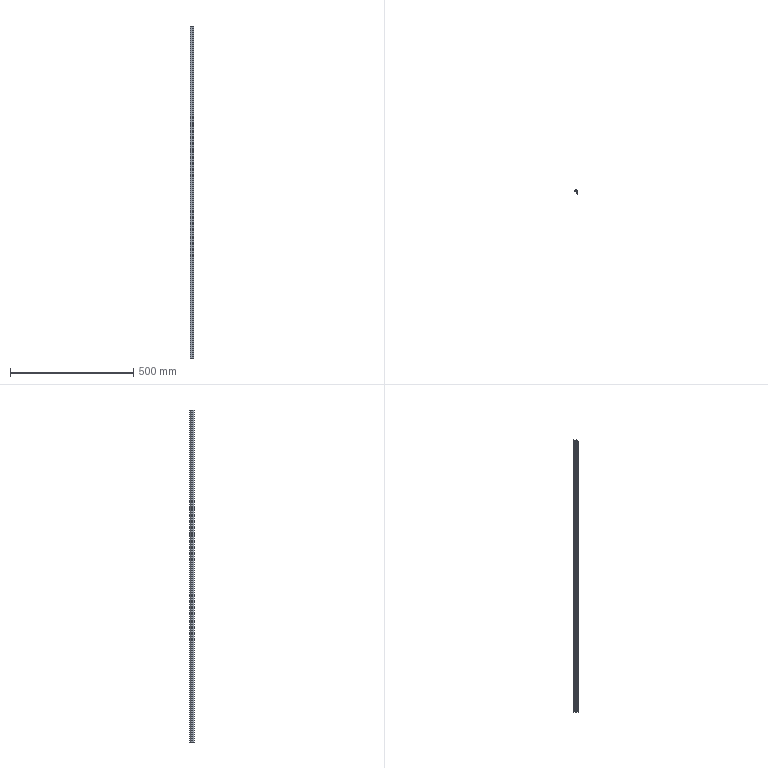Part | SolidWorks | features BaseBody 1, ICE 1, MoveFace 1 | 1 solid | 27 faces | box 14 x 20.3 x 1348 mm | volume 68634 mm3 | plane 20 | cylinder 7 | commonest cylinder face diameters 0.387 x2 0.8 x2 0.4 x1 20 x1 22 x1
STEP:
#1=CARTESIAN_POINT('',(-5.304,-0.625,200.));
#2=VERTEX_POINT('',#1);
#3=CARTESIAN_POINT('',(-5.449,-0.8125,200.));
#4=VERTEX_POINT('',#3);
#5=CARTESIAN_POINT('',(-5.255,-0.8125,200.));
#6=DIRECTION('',(0.,0.,1.));
#7=DIRECTION('',(-1.,0.,0.));
#8=AXIS2_PLACEMENT_3D('',#5,#6,#7);
#9=CIRCLE('',#8,0.1937);
#10=EDGE_CURVE('',#2,#4,#9,.T.);
#11=ORIENTED_EDGE('',*,*,#10,.T.);
#12=CARTESIAN_POINT('',(-5.449,-0.8125,-1148.));
#13=VERTEX_POINT('',#12);
#14=CARTESIAN_POINT('',(-5.449,-0.8125,230.));
#15=DIRECTION('',(0.,0.,-1.));
#16=VECTOR('',#15,1000.);
#17=LINE('',#14,#16);
#18=EDGE_CURVE('',#4,#13,#17,.T.);
#19=ORIENTED_EDGE('',*,*,#18,.T.);
#20=CARTESIAN_POINT('',(-5.304,-0.625,-1148.));
#21=VERTEX_POINT('',#20);
#22=CARTESIAN_POINT('',(-5.255,-0.8125,-1148.));
#23=DIRECTION('',(0.,0.,-1.));
#24=DIRECTION('',(1.,0.,0.));
#25=AXIS2_PLACEMENT_3D('',#22,#23,#24);
#26=CIRCLE('',#25,0.1937);
#27=EDGE_CURVE('',#13,#21,#26,.T.);
#28=ORIENTED_EDGE('',*,*,#27,.T.);
#29=CARTESIAN_POINT('',(-5.304,-0.625,230.));
#30=DIRECTION('',(0.,0.,-1.));
#31=VECTOR('',#30,1000.);
#32=LINE('',#29,#31);
#33=EDGE_CURVE('',#2,#21,#32,.T.);
#34=ORIENTED_EDGE('',*,*,#33,.F.);
#35=EDGE_LOOP('',(#11,#19,#28,#34));
#36=FACE_OUTER_BOUND('',#35,.T.);
#37=CARTESIAN_POINT('',(-5.255,-0.8125,230.));
#38=DIRECTION('',(0.,0.,-1.));
#39=DIRECTION('',(-1.,0.,0.));
#40=AXIS2_PLACEMENT_3D('',#37,#38,#39);
#41=CYLINDRICAL_SURFACE('',#40,0.1937);
#42=ADVANCED_FACE('',(#36),#41,.F.);
#43=CARTESIAN_POINT('',(5.,-1.,-1148.));
#44=VERTEX_POINT('',#43);
#45=CARTESIAN_POINT('',(5.,-14.3,-1148.));
#46=VERTEX_POINT('',#45);
#47=CARTESIAN_POINT('',(5.,29.623,-1148.));
#48=DIRECTION('',(0.,-1.,0.));
#49=VECTOR('',#48,1000.);
#50=LINE('',#47,#49);
#51=EDGE_CURVE('',#44,#46,#50,.T.);
#52=ORIENTED_EDGE('',*,*,#51,.F.);
#53=CARTESIAN_POINT('',(5.,-1.,200.));
#54=VERTEX_POINT('',#53);
#55=CARTESIAN_POINT('',(5.,-1.,230.));
#56=DIRECTION('',(0.,0.,-1.));
#57=VECTOR('',#56,1000.);
#58=LINE('',#55,#57);
#59=EDGE_CURVE('',#54,#44,#58,.T.);
#60=ORIENTED_EDGE('',*,*,#59,.F.);
#61=CARTESIAN_POINT('',(5.,-14.3,200.));
#62=VERTEX_POINT('',#61);
#63=CARTESIAN_POINT('',(5.,-14.3,200.));
#64=DIRECTION('',(0.,1.,0.));
#65=VECTOR('',#64,1000.);
#66=LINE('',#63,#65);
#67=EDGE_CURVE('',#62,#54,#66,.T.);
#68=ORIENTED_EDGE('',*,*,#67,.F.);
#69=CARTESIAN_POINT('',(5.,-14.3,230.));
#70=DIRECTION('',(0.,0.,1.));
#71=VECTOR('',#70,1000.);
#72=LINE('',#69,#71);
#73=EDGE_CURVE('',#46,#62,#72,.T.);
#74=ORIENTED_EDGE('',*,*,#73,.F.);
#75=EDGE_LOOP('',(#52,#60,#68,#74));
#76=FACE_OUTER_BOUND('',#75,.T.);
#77=CARTESIAN_POINT('',(5.,-14.3,230.));
#78=DIRECTION('',(-1.,0.,0.));
#79=DIRECTION('',(0.,0.,1.));
#80=AXIS2_PLACEMENT_3D('',#77,#78,#79);
#81=PLANE('',#80);
#82=ADVANCED_FACE('',(#76),#81,.F.);
#83=CARTESIAN_POINT('',(-9.,-2.,-1148.));
#84=VERTEX_POINT('',#83);
#85=CARTESIAN_POINT('',(-9.,-2.,200.));
#86=VERTEX_POINT('',#85);
#87=CARTESIAN_POINT('',(-9.,-2.,230.));
#88=DIRECTION('',(0.,0.,1.));
#89=VECTOR('',#88,1000.);
#90=LINE('',#87,#89);
#91=EDGE_CURVE('',#84,#86,#90,.T.);
#92=ORIENTED_EDGE('',*,*,#91,.F.);
#93=CARTESIAN_POINT('',(0.9,-2.,-1148.));
#94=VERTEX_POINT('',#93);
#95=CARTESIAN_POINT('',(5.,-2.,-1148.));
#96=DIRECTION('',(-1.,0.,0.));
#97=VECTOR('',#96,1000.);
#98=LINE('',#95,#97);
#99=EDGE_CURVE('',#94,#84,#98,.T.);
#100=ORIENTED_EDGE('',*,*,#99,.F.);
#101=CARTESIAN_POINT('',(0.9,-2.,200.));
#102=VERTEX_POINT('',#101);
#103=CARTESIAN_POINT('',(0.9,-2.,230.));
#104=DIRECTION('',(0.,0.,-1.));
#105=VECTOR('',#104,1000.);
#106=LINE('',#103,#105);
#107=EDGE_CURVE('',#102,#94,#106,.T.);
#108=ORIENTED_EDGE('',*,*,#107,.F.);
#109=CARTESIAN_POINT('',(5.,-2.,200.));
#110=DIRECTION('',(1.,0.,0.));
#111=VECTOR('',#110,1000.);
#112=LINE('',#109,#111);
#113=EDGE_CURVE('',#86,#102,#112,.T.);
#114=ORIENTED_EDGE('',*,*,#113,.F.);
#115=EDGE_LOOP('',(#92,#100,#108,#114));
#116=FACE_OUTER_BOUND('',#115,.T.);
#117=CARTESIAN_POINT('',(-9.,-2.,230.));
#118=DIRECTION('',(0.,1.,0.));
#119=DIRECTION('',(0.,0.,1.));
#120=AXIS2_PLACEMENT_3D('',#117,#118,#119);
#121=PLANE('',#120);
#122=ADVANCED_FACE('',(#116),#121,.F.);
#123=CARTESIAN_POINT('',(4.,-6.,200.));
#124=VERTEX_POINT('',#123);
#125=CARTESIAN_POINT('',(4.,-3.,200.));
#126=VERTEX_POINT('',#125);
#127=CARTESIAN_POINT('',(4.,29.623,200.));
#128=DIRECTION('',(0.,1.,0.));
#129=VECTOR('',#128,1000.);
#130=LINE('',#127,#129);
#131=EDGE_CURVE('',#124,#126,#130,.T.);
#132=ORIENTED_EDGE('',*,*,#131,.F.);
#133=CARTESIAN_POINT('',(1.,-6.,200.));
#134=VERTEX_POINT('',#133);
#135=CARTESIAN_POINT('',(5.,-6.,200.));
#136=DIRECTION('',(1.,0.,0.));
#137=VECTOR('',#136,1000.);
#138=LINE('',#135,#137);
#139=EDGE_CURVE('',#134,#124,#138,.T.);
#140=ORIENTED_EDGE('',*,*,#139,.F.);
#141=CARTESIAN_POINT('',(1.,-6.7,200.));
#142=VERTEX_POINT('',#141);
#143=CARTESIAN_POINT('',(1.,-6.,200.));
#144=DIRECTION('',(0.,-1.,0.));
#145=VECTOR('',#144,1000.);
#146=LINE('',#143,#145);
#147=EDGE_CURVE('',#134,#142,#146,.T.);
#148=ORIENTED_EDGE('',*,*,#147,.T.);
#149=CARTESIAN_POINT('',(-1.7,-6.7,200.));
#150=VERTEX_POINT('',#149);
#151=CARTESIAN_POINT('',(5.,-6.7,200.));
#152=DIRECTION('',(1.,0.,0.));
#153=VECTOR('',#152,1000.);
#154=LINE('',#151,#153);
#155=EDGE_CURVE('',#150,#142,#154,.T.);
#156=ORIENTED_EDGE('',*,*,#155,.F.);
#157=CARTESIAN_POINT('',(-1.7,-7.7,200.));
#158=VERTEX_POINT('',#157);
#159=CARTESIAN_POINT('',(-1.7,-6.7,200.));
#160=DIRECTION('',(0.,-1.,0.));
#161=VECTOR('',#160,1000.);
#162=LINE('',#159,#161);
#163=EDGE_CURVE('',#150,#158,#162,.T.);
#164=ORIENTED_EDGE('',*,*,#163,.T.);
#165=CARTESIAN_POINT('',(4.,-7.7,200.));
#166=VERTEX_POINT('',#165);
#167=CARTESIAN_POINT('',(5.,-7.7,200.));
#168=DIRECTION('',(-1.,0.,0.));
#169=VECTOR('',#168,1000.);
#170=LINE('',#167,#169);
#171=EDGE_CURVE('',#166,#158,#170,.T.);
#172=ORIENTED_EDGE('',*,*,#171,.F.);
#173=CARTESIAN_POINT('',(4.,-14.3,200.));
#174=VERTEX_POINT('',#173);
#175=CARTESIAN_POINT('',(4.,29.623,200.));
#176=DIRECTION('',(0.,1.,0.));
#177=VECTOR('',#176,1000.);
#178=LINE('',#175,#177);
#179=EDGE_CURVE('',#174,#166,#178,.T.);
#180=ORIENTED_EDGE('',*,*,#179,.F.);
#181=CARTESIAN_POINT('',(5.,-14.3,200.));
#182=DIRECTION('',(-1.,0.,0.));
#183=VECTOR('',#182,1000.);
#184=LINE('',#181,#183);
#185=EDGE_CURVE('',#62,#174,#184,.T.);
#186=ORIENTED_EDGE('',*,*,#185,.F.);
#187=ORIENTED_EDGE('',*,*,#67,.T.);
#188=CARTESIAN_POINT('',(-5.207,-1.,200.));
#189=VERTEX_POINT('',#188);
#190=CARTESIAN_POINT('',(5.,-1.,200.));
#191=DIRECTION('',(1.,0.,0.));
#192=VECTOR('',#191,1000.);
#193=LINE('',#190,#192);
#194=EDGE_CURVE('',#189,#54,#193,.T.);
#195=ORIENTED_EDGE('',*,*,#194,.F.);
#196=CARTESIAN_POINT('',(-5.255,-0.8125,200.));
#197=DIRECTION('',(0.,0.,1.));
#198=DIRECTION('',(-1.,0.,0.));
#199=AXIS2_PLACEMENT_3D('',#196,#197,#198);
#200=CIRCLE('',#199,0.1937);
#201=EDGE_CURVE('',#4,#189,#200,.T.);
#202=ORIENTED_EDGE('',*,*,#201,.F.);
#203=ORIENTED_EDGE('',*,*,#10,.F.);
#204=CARTESIAN_POINT('',(-1.368,3.063,200.));
#205=VERTEX_POINT('',#204);
#206=CARTESIAN_POINT('',(-10.628,9.,200.));
#207=DIRECTION('',(0.,0.,1.));
#208=DIRECTION('',(-1.,0.,0.));
#209=AXIS2_PLACEMENT_3D('',#206,#207,#208);
#210=CIRCLE('',#209,11.);
#211=EDGE_CURVE('',#2,#205,#210,.T.);
#212=ORIENTED_EDGE('',*,*,#211,.T.);
#213=CARTESIAN_POINT('',(-1.,2.955,200.));
#214=VERTEX_POINT('',#213);
#215=CARTESIAN_POINT('',(-1.2,2.955,200.));
#216=DIRECTION('',(0.,0.,1.));
#217=DIRECTION('',(-1.,0.,0.));
#218=AXIS2_PLACEMENT_3D('',#215,#216,#217);
#219=CIRCLE('',#218,0.2);
#220=EDGE_CURVE('',#214,#205,#219,.T.);
#221=ORIENTED_EDGE('',*,*,#220,.F.);
#222=CARTESIAN_POINT('',(-1.,1.5,200.));
#223=VERTEX_POINT('',#222);
#224=CARTESIAN_POINT('',(-1.,2.955,200.));
#225=DIRECTION('',(0.,1.,0.));
#226=VECTOR('',#225,1000.);
#227=LINE('',#224,#226);
#228=EDGE_CURVE('',#223,#214,#227,.T.);
#229=ORIENTED_EDGE('',*,*,#228,.F.);
#230=CARTESIAN_POINT('',(0.,1.5,200.));
#231=VERTEX_POINT('',#230);
#232=CARTESIAN_POINT('',(-1.,1.5,200.));
#233=DIRECTION('',(-1.,0.,0.));
#234=VECTOR('',#233,1000.);
#235=LINE('',#232,#234);
#236=EDGE_CURVE('',#231,#223,#235,.T.);
#237=ORIENTED_EDGE('',*,*,#236,.F.);
#238=CARTESIAN_POINT('',(0.,6.,200.));
#239=VERTEX_POINT('',#238);
#240=CARTESIAN_POINT('',(0.,1.5,200.));
#241=DIRECTION('',(0.,-1.,0.));
#242=VECTOR('',#241,1000.);
#243=LINE('',#240,#242);
#244=EDGE_CURVE('',#239,#231,#243,.T.);
#245=ORIENTED_EDGE('',*,*,#244,.F.);
#246=CARTESIAN_POINT('',(-0.8,6.,200.));
#247=VERTEX_POINT('',#246);
#248=CARTESIAN_POINT('',(0.,6.,200.));
#249=DIRECTION('',(1.,0.,0.));
#250=VECTOR('',#249,1000.);
#251=LINE('',#248,#250);
#252=EDGE_CURVE('',#247,#239,#251,.T.);
#253=ORIENTED_EDGE('',*,*,#252,.F.);
#254=CARTESIAN_POINT('',(-1.178,5.731,200.));
#255=VERTEX_POINT('',#254);
#256=CARTESIAN_POINT('',(-0.8,5.6,200.));
#257=DIRECTION('',(0.,0.,1.));
#258=DIRECTION('',(-1.,0.,0.));
#259=AXIS2_PLACEMENT_3D('',#256,#257,#258);
#260=CIRCLE('',#259,0.4);
#261=EDGE_CURVE('',#247,#255,#260,.T.);
#262=ORIENTED_EDGE('',*,*,#261,.T.);
#263=CARTESIAN_POINT('',(-8.678,-0.8077,200.));
#264=VERTEX_POINT('',#263);
#265=CARTESIAN_POINT('',(-10.628,9.,200.));
#266=DIRECTION('',(0.,0.,1.));
#267=DIRECTION('',(-1.,0.,0.));
#268=AXIS2_PLACEMENT_3D('',#265,#266,#267);
#269=CIRCLE('',#268,10.);
#270=EDGE_CURVE('',#264,#255,#269,.T.);
#271=ORIENTED_EDGE('',*,*,#270,.F.);
#272=CARTESIAN_POINT('',(-9.,-1.2,200.));
#273=VERTEX_POINT('',#272);
#274=CARTESIAN_POINT('',(-8.6,-1.2,200.));
#275=DIRECTION('',(0.,0.,1.));
#276=DIRECTION('',(-1.,0.,0.));
#277=AXIS2_PLACEMENT_3D('',#274,#275,#276);
#278=CIRCLE('',#277,0.4);
#279=EDGE_CURVE('',#264,#273,#278,.T.);
#280=ORIENTED_EDGE('',*,*,#279,.T.);
#281=CARTESIAN_POINT('',(-9.,8.,200.));
#282=DIRECTION('',(0.,-1.,0.));
#283=VECTOR('',#282,1000.);
#284=LINE('',#281,#283);
#285=EDGE_CURVE('',#273,#86,#284,.T.);
#286=ORIENTED_EDGE('',*,*,#285,.T.);
#287=ORIENTED_EDGE('',*,*,#113,.T.);
#288=CARTESIAN_POINT('',(0.9,-3.,200.));
#289=VERTEX_POINT('',#288);
#290=CARTESIAN_POINT('',(0.9,29.623,200.));
#291=DIRECTION('',(0.,1.,0.));
#292=VECTOR('',#291,1000.);
#293=LINE('',#290,#292);
#294=EDGE_CURVE('',#289,#102,#293,.T.);
#295=ORIENTED_EDGE('',*,*,#294,.F.);
#296=CARTESIAN_POINT('',(5.,-3.,200.));
#297=DIRECTION('',(-1.,0.,0.));
#298=VECTOR('',#297,1000.);
#299=LINE('',#296,#298);
#300=EDGE_CURVE('',#126,#289,#299,.T.);
#301=ORIENTED_EDGE('',*,*,#300,.F.);
#302=EDGE_LOOP('',(#132,#140,#148,#156,#164,#172,#180,#186,#187,#195,#202,#203,#212,#221,#229,#237,#245,#253,#262,#271,#280,#286,#287,#295,#301));
#303=FACE_OUTER_BOUND('',#302,.T.);
#304=CARTESIAN_POINT('',(5.,29.623,200.));
#305=DIRECTION('',(0.,0.,-1.));
#306=DIRECTION('',(-1.,0.,0.));
#307=AXIS2_PLACEMENT_3D('',#304,#305,#306);
#308=PLANE('',#307);
#309=ADVANCED_FACE('',(#303),#308,.F.);
#310=ORIENTED_EDGE('',*,*,#185,.T.);
#311=CARTESIAN_POINT('',(4.,-14.3,-1148.));
#312=VERTEX_POINT('',#311);
#313=CARTESIAN_POINT('',(4.,-14.3,230.));
#314=DIRECTION('',(0.,0.,1.));
#315=VECTOR('',#314,1000.);
#316=LINE('',#313,#315);
#317=EDGE_CURVE('',#312,#174,#316,.T.);
#318=ORIENTED_EDGE('',*,*,#317,.F.);
#319=CARTESIAN_POINT('',(5.,-14.3,-1148.));
#320=DIRECTION('',(-1.,0.,0.));
#321=VECTOR('',#320,1000.);
#322=LINE('',#319,#321);
#323=EDGE_CURVE('',#46,#312,#322,.T.);
#324=ORIENTED_EDGE('',*,*,#323,.F.);
#325=ORIENTED_EDGE('',*,*,#73,.T.);
#326=EDGE_LOOP('',(#310,#318,#324,#325));
#327=FACE_OUTER_BOUND('',#326,.T.);
#328=CARTESIAN_POINT('',(4.,-14.3,230.));
#329=DIRECTION('',(0.,1.,0.));
#330=DIRECTION('',(0.,0.,1.));
#331=AXIS2_PLACEMENT_3D('',#328,#329,#330);
#332=PLANE('',#331);
#333=ADVANCED_FACE('',(#327),#332,.F.);
#334=ORIENTED_EDGE('',*,*,#51,.T.);
#335=ORIENTED_EDGE('',*,*,#323,.T.);
#336=CARTESIAN_POINT('',(4.,-7.7,-1148.));
#337=VERTEX_POINT('',#336);
#338=CARTESIAN_POINT('',(4.,-7.7,-1148.));
#339=DIRECTION('',(0.,-1.,0.));
#340=VECTOR('',#339,1000.);
#341=LINE('',#338,#340);
#342=EDGE_CURVE('',#337,#312,#341,.T.);
#343=ORIENTED_EDGE('',*,*,#342,.F.);
#344=CARTESIAN_POINT('',(-1.7,-7.7,-1148.));
#345=VERTEX_POINT('',#344);
#346=CARTESIAN_POINT('',(-1.7,-7.7,-1148.));
#347=DIRECTION('',(1.,0.,0.));
#348=VECTOR('',#347,1000.);
#349=LINE('',#346,#348);
#350=EDGE_CURVE('',#345,#337,#349,.T.);
#351=ORIENTED_EDGE('',*,*,#350,.F.);
#352=CARTESIAN_POINT('',(-1.7,-6.7,-1148.));
#353=VERTEX_POINT('',#352);
#354=CARTESIAN_POINT('',(-1.7,29.623,-1148.));
#355=DIRECTION('',(0.,1.,0.));
#356=VECTOR('',#355,1000.);
#357=LINE('',#354,#356);
#358=EDGE_CURVE('',#345,#353,#357,.T.);
#359=ORIENTED_EDGE('',*,*,#358,.T.);
#360=CARTESIAN_POINT('',(1.,-6.7,-1148.));
#361=VERTEX_POINT('',#360);
#362=CARTESIAN_POINT('',(1.,-6.7,-1148.));
#363=DIRECTION('',(-1.,0.,0.));
#364=VECTOR('',#363,1000.);
#365=LINE('',#362,#364);
#366=EDGE_CURVE('',#361,#353,#365,.T.);
#367=ORIENTED_EDGE('',*,*,#366,.F.);
#368=CARTESIAN_POINT('',(1.,-6.,-1148.));
#369=VERTEX_POINT('',#368);
#370=CARTESIAN_POINT('',(1.,29.623,-1148.));
#371=DIRECTION('',(0.,1.,0.));
#372=VECTOR('',#371,1000.);
#373=LINE('',#370,#372);
#374=EDGE_CURVE('',#361,#369,#373,.T.);
#375=ORIENTED_EDGE('',*,*,#374,.T.);
#376=CARTESIAN_POINT('',(4.,-6.,-1148.));
#377=VERTEX_POINT('',#376);
#378=CARTESIAN_POINT('',(4.,-6.,-1148.));
#379=DIRECTION('',(-1.,0.,0.));
#380=VECTOR('',#379,1000.);
#381=LINE('',#378,#380);
#382=EDGE_CURVE('',#377,#369,#381,.T.);
#383=ORIENTED_EDGE('',*,*,#382,.F.);
#384=CARTESIAN_POINT('',(4.,-3.,-1148.));
#385=VERTEX_POINT('',#384);
#386=CARTESIAN_POINT('',(4.,-3.,-1148.));
#387=DIRECTION('',(0.,-1.,0.));
#388=VECTOR('',#387,1000.);
#389=LINE('',#386,#388);
#390=EDGE_CURVE('',#385,#377,#389,.T.);
#391=ORIENTED_EDGE('',*,*,#390,.F.);
#392=CARTESIAN_POINT('',(0.9,-3.,-1148.));
#393=VERTEX_POINT('',#392);
#394=CARTESIAN_POINT('',(0.9,-3.,-1148.));
#395=DIRECTION('',(1.,0.,0.));
#396=VECTOR('',#395,1000.);
#397=LINE('',#394,#396);
#398=EDGE_CURVE('',#393,#385,#397,.T.);
#399=ORIENTED_EDGE('',*,*,#398,.F.);
#400=CARTESIAN_POINT('',(0.9,-2.,-1148.));
#401=DIRECTION('',(0.,-1.,0.));
#402=VECTOR('',#401,1000.);
#403=LINE('',#400,#402);
#404=EDGE_CURVE('',#94,#393,#403,.T.);
#405=ORIENTED_EDGE('',*,*,#404,.F.);
#406=ORIENTED_EDGE('',*,*,#99,.T.);
#407=CARTESIAN_POINT('',(-9.,-1.2,-1148.));
#408=VERTEX_POINT('',#407);
#409=CARTESIAN_POINT('',(-9.,-1.2,-1148.));
#410=DIRECTION('',(0.,-1.,0.));
#411=VECTOR('',#410,1000.);
#412=LINE('',#409,#411);
#413=EDGE_CURVE('',#408,#84,#412,.T.);
#414=ORIENTED_EDGE('',*,*,#413,.F.);
#415=CARTESIAN_POINT('',(-8.678,-0.8077,-1148.));
#416=VERTEX_POINT('',#415);
#417=CARTESIAN_POINT('',(-8.6,-1.2,-1148.));
#418=DIRECTION('',(0.,0.,-1.));
#419=DIRECTION('',(1.,0.,0.));
#420=AXIS2_PLACEMENT_3D('',#417,#418,#419);
#421=CIRCLE('',#420,0.4);
#422=EDGE_CURVE('',#408,#416,#421,.T.);
#423=ORIENTED_EDGE('',*,*,#422,.T.);
#424=CARTESIAN_POINT('',(-1.178,5.731,-1148.));
#425=VERTEX_POINT('',#424);
#426=CARTESIAN_POINT('',(-10.628,9.,-1148.));
#427=DIRECTION('',(0.,0.,-1.));
#428=DIRECTION('',(1.,0.,0.));
#429=AXIS2_PLACEMENT_3D('',#426,#427,#428);
#430=CIRCLE('',#429,10.);
#431=EDGE_CURVE('',#425,#416,#430,.T.);
#432=ORIENTED_EDGE('',*,*,#431,.F.);
#433=CARTESIAN_POINT('',(-0.8,6.,-1148.));
#434=VERTEX_POINT('',#433);
#435=CARTESIAN_POINT('',(-0.8,5.6,-1148.));
#436=DIRECTION('',(0.,0.,-1.));
#437=DIRECTION('',(1.,0.,0.));
#438=AXIS2_PLACEMENT_3D('',#435,#436,#437);
#439=CIRCLE('',#438,0.4);
#440=EDGE_CURVE('',#425,#434,#439,.T.);
#441=ORIENTED_EDGE('',*,*,#440,.T.);
#442=CARTESIAN_POINT('',(0.,6.,-1148.));
#443=VERTEX_POINT('',#442);
#444=CARTESIAN_POINT('',(0.,6.,-1148.));
#445=DIRECTION('',(-1.,0.,0.));
#446=VECTOR('',#445,1000.);
#447=LINE('',#444,#446);
#448=EDGE_CURVE('',#443,#434,#447,.T.);
#449=ORIENTED_EDGE('',*,*,#448,.F.);
#450=CARTESIAN_POINT('',(0.,1.5,-1148.));
#451=VERTEX_POINT('',#450);
#452=CARTESIAN_POINT('',(0.,1.5,-1148.));
#453=DIRECTION('',(0.,1.,0.));
#454=VECTOR('',#453,1000.);
#455=LINE('',#452,#454);
#456=EDGE_CURVE('',#451,#443,#455,.T.);
#457=ORIENTED_EDGE('',*,*,#456,.F.);
#458=CARTESIAN_POINT('',(-1.,1.5,-1148.));
#459=VERTEX_POINT('',#458);
#460=CARTESIAN_POINT('',(-1.,1.5,-1148.));
#461=DIRECTION('',(1.,0.,0.));
#462=VECTOR('',#461,1000.);
#463=LINE('',#460,#462);
#464=EDGE_CURVE('',#459,#451,#463,.T.);
#465=ORIENTED_EDGE('',*,*,#464,.F.);
#466=CARTESIAN_POINT('',(-1.,2.955,-1148.));
#467=VERTEX_POINT('',#466);
#468=CARTESIAN_POINT('',(-1.,2.955,-1148.));
#469=DIRECTION('',(0.,-1.,0.));
#470=VECTOR('',#469,1000.);
#471=LINE('',#468,#470);
#472=EDGE_CURVE('',#467,#459,#471,.T.);
#473=ORIENTED_EDGE('',*,*,#472,.F.);
#474=CARTESIAN_POINT('',(-1.368,3.063,-1148.));
#475=VERTEX_POINT('',#474);
#476=CARTESIAN_POINT('',(-1.2,2.955,-1148.));
#477=DIRECTION('',(0.,0.,-1.));
#478=DIRECTION('',(1.,0.,0.));
#479=AXIS2_PLACEMENT_3D('',#476,#477,#478);
#480=CIRCLE('',#479,0.2);
#481=EDGE_CURVE('',#475,#467,#480,.T.);
#482=ORIENTED_EDGE('',*,*,#481,.F.);
#483=CARTESIAN_POINT('',(-10.628,9.,-1148.));
#484=DIRECTION('',(0.,0.,-1.));
#485=DIRECTION('',(1.,0.,0.));
#486=AXIS2_PLACEMENT_3D('',#483,#484,#485);
#487=CIRCLE('',#486,11.);
#488=EDGE_CURVE('',#475,#21,#487,.T.);
#489=ORIENTED_EDGE('',*,*,#488,.T.);
#490=ORIENTED_EDGE('',*,*,#27,.F.);
#491=CARTESIAN_POINT('',(-5.207,-1.,-1148.));
#492=VERTEX_POINT('',#491);
#493=CARTESIAN_POINT('',(-5.255,-0.8125,-1148.));
#494=DIRECTION('',(0.,0.,-1.));
#495=DIRECTION('',(1.,0.,0.));
#496=AXIS2_PLACEMENT_3D('',#493,#494,#495);
#497=CIRCLE('',#496,0.1937);
#498=EDGE_CURVE('',#492,#13,#497,.T.);
#499=ORIENTED_EDGE('',*,*,#498,.F.);
#500=CARTESIAN_POINT('',(5.,-1.,-1148.));
#501=DIRECTION('',(-1.,0.,0.));
#502=VECTOR('',#501,1000.);
#503=LINE('',#500,#502);
#504=EDGE_CURVE('',#44,#492,#503,.T.);
#505=ORIENTED_EDGE('',*,*,#504,.F.);
#506=EDGE_LOOP('',(#334,#335,#343,#351,#359,#367,#375,#383,#391,#399,#405,#406,#414,#423,#432,#441,#449,#457,#465,#473,#482,#489,#490,#499,#505));
#507=FACE_OUTER_BOUND('',#506,.T.);
#508=CARTESIAN_POINT('',(5.,29.623,-1148.));
#509=DIRECTION('',(0.,0.,1.));
#510=DIRECTION('',(1.,0.,0.));
#511=AXIS2_PLACEMENT_3D('',#508,#509,#510);
#512=PLANE('',#511);
#513=ADVANCED_FACE('',(#507),#512,.F.);
#514=ORIENTED_EDGE('',*,*,#59,.T.);
#515=ORIENTED_EDGE('',*,*,#504,.T.);
#516=CARTESIAN_POINT('',(-5.207,-1.,230.));
#517=DIRECTION('',(0.,0.,-1.));
#518=VECTOR('',#517,1000.);
#519=LINE('',#516,#518);
#520=EDGE_CURVE('',#189,#492,#519,.T.);
#521=ORIENTED_EDGE('',*,*,#520,.F.);
#522=ORIENTED_EDGE('',*,*,#194,.T.);
#523=EDGE_LOOP('',(#514,#515,#521,#522));
#524=FACE_OUTER_BOUND('',#523,.T.);
#525=CARTESIAN_POINT('',(5.,-1.,230.));
#526=DIRECTION('',(0.,-1.,0.));
#527=DIRECTION('',(0.,0.,-1.));
#528=AXIS2_PLACEMENT_3D('',#525,#526,#527);
#529=PLANE('',#528);
#530=ADVANCED_FACE('',(#524),#529,.F.);
#531=CARTESIAN_POINT('',(-9.,-1.2,230.));
#532=DIRECTION('',(0.,0.,1.));
#533=VECTOR('',#532,1000.);
#534=LINE('',#531,#533);
#535=EDGE_CURVE('',#408,#273,#534,.T.);
#536=ORIENTED_EDGE('',*,*,#535,.F.);
#537=ORIENTED_EDGE('',*,*,#413,.T.);
#538=ORIENTED_EDGE('',*,*,#91,.T.);
#539=ORIENTED_EDGE('',*,*,#285,.F.);
#540=EDGE_LOOP('',(#536,#537,#538,#539));
#541=FACE_OUTER_BOUND('',#540,.T.);
#542=CARTESIAN_POINT('',(-9.,-1.2,230.));
#543=DIRECTION('',(1.,0.,0.));
#544=DIRECTION('',(0.,0.,-1.));
#545=AXIS2_PLACEMENT_3D('',#542,#543,#544);
#546=PLANE('',#545);
#547=ADVANCED_FACE('',(#541),#546,.F.);
#548=ORIENTED_EDGE('',*,*,#294,.T.);
#549=ORIENTED_EDGE('',*,*,#107,.T.);
#550=ORIENTED_EDGE('',*,*,#404,.T.);
#551=CARTESIAN_POINT('',(0.9,-3.,230.));
#552=DIRECTION('',(0.,0.,-1.));
#553=VECTOR('',#552,1000.);
#554=LINE('',#551,#553);
#555=EDGE_CURVE('',#289,#393,#554,.T.);
#556=ORIENTED_EDGE('',*,*,#555,.F.);
#557=EDGE_LOOP('',(#548,#549,#550,#556));
#558=FACE_OUTER_BOUND('',#557,.T.);
#559=CARTESIAN_POINT('',(0.9,-2.,230.));
#560=DIRECTION('',(1.,0.,0.));
#561=DIRECTION('',(0.,0.,-1.));
#562=AXIS2_PLACEMENT_3D('',#559,#560,#561);
#563=PLANE('',#562);
#564=ADVANCED_FACE('',(#558),#563,.F.);
#565=ORIENTED_EDGE('',*,*,#300,.T.);
#566=ORIENTED_EDGE('',*,*,#555,.T.);
#567=ORIENTED_EDGE('',*,*,#398,.T.);
#568=CARTESIAN_POINT('',(4.,-3.,230.));
#569=DIRECTION('',(0.,0.,-1.));
#570=VECTOR('',#569,1000.);
#571=LINE('',#568,#570);
#572=EDGE_CURVE('',#126,#385,#571,.T.);
#573=ORIENTED_EDGE('',*,*,#572,.F.);
#574=EDGE_LOOP('',(#565,#566,#567,#573));
#575=FACE_OUTER_BOUND('',#574,.T.);
#576=CARTESIAN_POINT('',(0.9,-3.,230.));
#577=DIRECTION('',(0.,1.,0.));
#578=DIRECTION('',(0.,0.,1.));
#579=AXIS2_PLACEMENT_3D('',#576,#577,#578);
#580=PLANE('',#579);
#581=ADVANCED_FACE('',(#575),#580,.F.);
#582=ORIENTED_EDGE('',*,*,#131,.T.);
#583=ORIENTED_EDGE('',*,*,#572,.T.);
#584=ORIENTED_EDGE('',*,*,#390,.T.);
#585=CARTESIAN_POINT('',(4.,-6.,230.));
#586=DIRECTION('',(0.,0.,-1.));
#587=VECTOR('',#586,1000.);
#588=LINE('',#585,#587);
#589=EDGE_CURVE('',#124,#377,#588,.T.);
#590=ORIENTED_EDGE('',*,*,#589,.F.);
#591=EDGE_LOOP('',(#582,#583,#584,#590));
#592=FACE_OUTER_BOUND('',#591,.T.);
#593=CARTESIAN_POINT('',(4.,-3.,230.));
#594=DIRECTION('',(1.,0.,0.));
#595=DIRECTION('',(0.,0.,-1.));
#596=AXIS2_PLACEMENT_3D('',#593,#594,#595);
#597=PLANE('',#596);
#598=ADVANCED_FACE('',(#592),#597,.F.);
#599=ORIENTED_EDGE('',*,*,#139,.T.);
#600=ORIENTED_EDGE('',*,*,#589,.T.);
#601=ORIENTED_EDGE('',*,*,#382,.T.);
#602=CARTESIAN_POINT('',(1.,-6.,230.));
#603=DIRECTION('',(0.,0.,-1.));
#604=VECTOR('',#603,1000.);
#605=LINE('',#602,#604);
#606=EDGE_CURVE('',#134,#369,#605,.T.);
#607=ORIENTED_EDGE('',*,*,#606,.F.);
#608=EDGE_LOOP('',(#599,#600,#601,#607));
#609=FACE_OUTER_BOUND('',#608,.T.);
#610=CARTESIAN_POINT('',(4.,-6.,230.));
#611=DIRECTION('',(0.,-1.,0.));
#612=DIRECTION('',(0.,0.,-1.));
#613=AXIS2_PLACEMENT_3D('',#610,#611,#612);
#614=PLANE('',#613);
#615=ADVANCED_FACE('',(#609),#614,.F.);
#616=ORIENTED_EDGE('',*,*,#155,.T.);
#617=CARTESIAN_POINT('',(1.,-6.7,230.));
#618=DIRECTION('',(0.,0.,1.));
#619=VECTOR('',#618,1000.);
#620=LINE('',#617,#619);
#621=EDGE_CURVE('',#361,#142,#620,.T.);
#622=ORIENTED_EDGE('',*,*,#621,.F.);
#623=ORIENTED_EDGE('',*,*,#366,.T.);
#624=CARTESIAN_POINT('',(-1.7,-6.7,230.));
#625=DIRECTION('',(0.,0.,-1.));
#626=VECTOR('',#625,1000.);
#627=LINE('',#624,#626);
#628=EDGE_CURVE('',#150,#353,#627,.T.);
#629=ORIENTED_EDGE('',*,*,#628,.F.);
#630=EDGE_LOOP('',(#616,#622,#623,#629));
#631=FACE_OUTER_BOUND('',#630,.T.);
#632=CARTESIAN_POINT('',(1.,-6.7,230.));
#633=DIRECTION('',(0.,-1.,0.));
#634=DIRECTION('',(0.,0.,-1.));
#635=AXIS2_PLACEMENT_3D('',#632,#633,#634);
#636=PLANE('',#635);
#637=ADVANCED_FACE('',(#631),#636,.F.);
#638=ORIENTED_EDGE('',*,*,#171,.T.);
#639=CARTESIAN_POINT('',(-1.7,-7.7,230.));
#640=DIRECTION('',(0.,0.,1.));
#641=VECTOR('',#640,1000.);
#642=LINE('',#639,#641);
#643=EDGE_CURVE('',#345,#158,#642,.T.);
#644=ORIENTED_EDGE('',*,*,#643,.F.);
#645=ORIENTED_EDGE('',*,*,#350,.T.);
#646=CARTESIAN_POINT('',(4.,-7.7,230.));
#647=DIRECTION('',(0.,0.,-1.));
#648=VECTOR('',#647,1000.);
#649=LINE('',#646,#648);
#650=EDGE_CURVE('',#166,#337,#649,.T.);
#651=ORIENTED_EDGE('',*,*,#650,.F.);
#652=EDGE_LOOP('',(#638,#644,#645,#651));
#653=FACE_OUTER_BOUND('',#652,.T.);
#654=CARTESIAN_POINT('',(-1.7,-7.7,230.));
#655=DIRECTION('',(0.,1.,0.));
#656=DIRECTION('',(0.,0.,1.));
#657=AXIS2_PLACEMENT_3D('',#654,#655,#656);
#658=PLANE('',#657);
#659=ADVANCED_FACE('',(#653),#658,.F.);
#660=ORIENTED_EDGE('',*,*,#179,.T.);
#661=ORIENTED_EDGE('',*,*,#650,.T.);
#662=ORIENTED_EDGE('',*,*,#342,.T.);
#663=ORIENTED_EDGE('',*,*,#317,.T.);
#664=EDGE_LOOP('',(#660,#661,#662,#663));
#665=FACE_OUTER_BOUND('',#664,.T.);
#666=CARTESIAN_POINT('',(4.,-7.7,230.));
#667=DIRECTION('',(1.,0.,0.));
#668=DIRECTION('',(0.,0.,-1.));
#669=AXIS2_PLACEMENT_3D('',#666,#667,#668);
#670=PLANE('',#669);
#671=ADVANCED_FACE('',(#665),#670,.F.);
#672=ORIENTED_EDGE('',*,*,#18,.F.);
#673=ORIENTED_EDGE('',*,*,#201,.T.);
#674=ORIENTED_EDGE('',*,*,#520,.T.);
#675=ORIENTED_EDGE('',*,*,#498,.T.);
#676=EDGE_LOOP('',(#672,#673,#674,#675));
#677=FACE_OUTER_BOUND('',#676,.T.);
#678=CARTESIAN_POINT('',(-5.255,-0.8125,230.));
#679=DIRECTION('',(0.,0.,-1.));
#680=DIRECTION('',(-1.,0.,0.));
#681=AXIS2_PLACEMENT_3D('',#678,#679,#680);
#682=CYLINDRICAL_SURFACE('',#681,0.1937);
#683=ADVANCED_FACE('',(#677),#682,.F.);
#684=CARTESIAN_POINT('',(-1.,2.955,230.));
#685=DIRECTION('',(0.,0.,1.));
#686=VECTOR('',#685,1000.);
#687=LINE('',#684,#686);
#688=EDGE_CURVE('',#467,#214,#687,.T.);
#689=ORIENTED_EDGE('',*,*,#688,.F.);
#690=ORIENTED_EDGE('',*,*,#472,.T.);
#691=CARTESIAN_POINT('',(-1.,1.5,230.));
#692=DIRECTION('',(0.,0.,-1.));
#693=VECTOR('',#692,1000.);
#694=LINE('',#691,#693);
#695=EDGE_CURVE('',#223,#459,#694,.T.);
#696=ORIENTED_EDGE('',*,*,#695,.F.);
#697=ORIENTED_EDGE('',*,*,#228,.T.);
#698=EDGE_LOOP('',(#689,#690,#696,#697));
#699=FACE_OUTER_BOUND('',#698,.T.);
#700=CARTESIAN_POINT('',(-1.,2.955,230.));
#701=DIRECTION('',(1.,0.,0.));
#702=DIRECTION('',(0.,0.,-1.));
#703=AXIS2_PLACEMENT_3D('',#700,#701,#702);
#704=PLANE('',#703);
#705=ADVANCED_FACE('',(#699),#704,.F.);
#706=ORIENTED_EDGE('',*,*,#488,.F.);
#707=CARTESIAN_POINT('',(-1.368,3.063,230.));
#708=DIRECTION('',(0.,0.,1.));
#709=VECTOR('',#708,1000.);
#710=LINE('',#707,#709);
#711=EDGE_CURVE('',#475,#205,#710,.T.);
#712=ORIENTED_EDGE('',*,*,#711,.T.);
#713=ORIENTED_EDGE('',*,*,#211,.F.);
#714=ORIENTED_EDGE('',*,*,#33,.T.);
#715=EDGE_LOOP('',(#706,#712,#713,#714));
#716=FACE_OUTER_BOUND('',#715,.T.);
#717=CARTESIAN_POINT('',(-10.628,9.,230.));
#718=DIRECTION('',(0.,0.,-1.));
#719=DIRECTION('',(-1.,0.,0.));
#720=AXIS2_PLACEMENT_3D('',#717,#718,#719);
#721=CYLINDRICAL_SURFACE('',#720,11.);
#722=ADVANCED_FACE('',(#716),#721,.T.);
#723=CARTESIAN_POINT('',(-1.178,5.731,230.));
#724=DIRECTION('',(0.,0.,1.));
#725=VECTOR('',#724,1000.);
#726=LINE('',#723,#725);
#727=EDGE_CURVE('',#425,#255,#726,.T.);
#728=ORIENTED_EDGE('',*,*,#727,.F.);
#729=ORIENTED_EDGE('',*,*,#431,.T.);
#730=CARTESIAN_POINT('',(-8.678,-0.8077,230.));
#731=DIRECTION('',(0.,0.,-1.));
#732=VECTOR('',#731,1000.);
#733=LINE('',#730,#732);
#734=EDGE_CURVE('',#264,#416,#733,.T.);
#735=ORIENTED_EDGE('',*,*,#734,.F.);
#736=ORIENTED_EDGE('',*,*,#270,.T.);
#737=EDGE_LOOP('',(#728,#729,#735,#736));
#738=FACE_OUTER_BOUND('',#737,.T.);
#739=CARTESIAN_POINT('',(-10.628,9.,230.));
#740=DIRECTION('',(0.,0.,-1.));
#741=DIRECTION('',(-1.,0.,0.));
#742=AXIS2_PLACEMENT_3D('',#739,#740,#741);
#743=CYLINDRICAL_SURFACE('',#742,10.);
#744=ADVANCED_FACE('',(#738),#743,.F.);
#745=CARTESIAN_POINT('',(0.,1.5,230.));
#746=DIRECTION('',(0.,0.,1.));
#747=VECTOR('',#746,1000.);
#748=LINE('',#745,#747);
#749=EDGE_CURVE('',#451,#231,#748,.T.);
#750=ORIENTED_EDGE('',*,*,#749,.F.);
#751=ORIENTED_EDGE('',*,*,#456,.T.);
#752=CARTESIAN_POINT('',(0.,6.,230.));
#753=DIRECTION('',(0.,0.,-1.));
#754=VECTOR('',#753,1000.);
#755=LINE('',#752,#754);
#756=EDGE_CURVE('',#239,#443,#755,.T.);
#757=ORIENTED_EDGE('',*,*,#756,.F.);
#758=ORIENTED_EDGE('',*,*,#244,.T.);
#759=EDGE_LOOP('',(#750,#751,#757,#758));
#760=FACE_OUTER_BOUND('',#759,.T.);
#761=CARTESIAN_POINT('',(0.,1.5,230.));
#762=DIRECTION('',(-1.,0.,0.));
#763=DIRECTION('',(0.,0.,1.));
#764=AXIS2_PLACEMENT_3D('',#761,#762,#763);
#765=PLANE('',#764);
#766=ADVANCED_FACE('',(#760),#765,.F.);
#767=ORIENTED_EDGE('',*,*,#422,.F.);
#768=ORIENTED_EDGE('',*,*,#535,.T.);
#769=ORIENTED_EDGE('',*,*,#279,.F.);
#770=ORIENTED_EDGE('',*,*,#734,.T.);
#771=EDGE_LOOP('',(#767,#768,#769,#770));
#772=FACE_OUTER_BOUND('',#771,.T.);
#773=CARTESIAN_POINT('',(-8.6,-1.2,230.));
#774=DIRECTION('',(0.,0.,-1.));
#775=DIRECTION('',(-1.,0.,0.));
#776=AXIS2_PLACEMENT_3D('',#773,#774,#775);
#777=CYLINDRICAL_SURFACE('',#776,0.4);
#778=ADVANCED_FACE('',(#772),#777,.T.);
#779=ORIENTED_EDGE('',*,*,#147,.F.);
#780=ORIENTED_EDGE('',*,*,#606,.T.);
#781=ORIENTED_EDGE('',*,*,#374,.F.);
#782=ORIENTED_EDGE('',*,*,#621,.T.);
#783=EDGE_LOOP('',(#779,#780,#781,#782));
#784=FACE_OUTER_BOUND('',#783,.T.);
#785=CARTESIAN_POINT('',(1.,-6.,230.));
#786=DIRECTION('',(1.,0.,0.));
#787=DIRECTION('',(0.,0.,-1.));
#788=AXIS2_PLACEMENT_3D('',#785,#786,#787);
#789=PLANE('',#788);
#790=ADVANCED_FACE('',(#784),#789,.F.);
#791=ORIENTED_EDGE('',*,*,#163,.F.);
#792=ORIENTED_EDGE('',*,*,#628,.T.);
#793=ORIENTED_EDGE('',*,*,#358,.F.);
#794=ORIENTED_EDGE('',*,*,#643,.T.);
#795=EDGE_LOOP('',(#791,#792,#793,#794));
#796=FACE_OUTER_BOUND('',#795,.T.);
#797=CARTESIAN_POINT('',(-1.7,-6.7,230.));
#798=DIRECTION('',(1.,0.,0.));
#799=DIRECTION('',(0.,0.,-1.));
#800=AXIS2_PLACEMENT_3D('',#797,#798,#799);
#801=PLANE('',#800);
#802=ADVANCED_FACE('',(#796),#801,.F.);
#803=ORIENTED_EDGE('',*,*,#711,.F.);
#804=ORIENTED_EDGE('',*,*,#481,.T.);
#805=ORIENTED_EDGE('',*,*,#688,.T.);
#806=ORIENTED_EDGE('',*,*,#220,.T.);
#807=EDGE_LOOP('',(#803,#804,#805,#806));
#808=FACE_OUTER_BOUND('',#807,.T.);
#809=CARTESIAN_POINT('',(-1.2,2.955,230.));
#810=DIRECTION('',(0.,0.,-1.));
#811=DIRECTION('',(-1.,0.,0.));
#812=AXIS2_PLACEMENT_3D('',#809,#810,#811);
#813=CYLINDRICAL_SURFACE('',#812,0.2);
#814=ADVANCED_FACE('',(#808),#813,.F.);
#815=ORIENTED_EDGE('',*,*,#695,.T.);
#816=ORIENTED_EDGE('',*,*,#464,.T.);
#817=ORIENTED_EDGE('',*,*,#749,.T.);
#818=ORIENTED_EDGE('',*,*,#236,.T.);
#819=EDGE_LOOP('',(#815,#816,#817,#818));
#820=FACE_OUTER_BOUND('',#819,.T.);
#821=CARTESIAN_POINT('',(-1.,1.5,230.));
#822=DIRECTION('',(0.,1.,0.));
#823=DIRECTION('',(0.,0.,1.));
#824=AXIS2_PLACEMENT_3D('',#821,#822,#823);
#825=PLANE('',#824);
#826=ADVANCED_FACE('',(#820),#825,.F.);
#827=ORIENTED_EDGE('',*,*,#440,.F.);
#828=ORIENTED_EDGE('',*,*,#727,.T.);
#829=ORIENTED_EDGE('',*,*,#261,.F.);
#830=CARTESIAN_POINT('',(-0.8,6.,230.));
#831=DIRECTION('',(0.,0.,-1.));
#832=VECTOR('',#831,1000.);
#833=LINE('',#830,#832);
#834=EDGE_CURVE('',#247,#434,#833,.T.);
#835=ORIENTED_EDGE('',*,*,#834,.T.);
#836=EDGE_LOOP('',(#827,#828,#829,#835));
#837=FACE_OUTER_BOUND('',#836,.T.);
#838=CARTESIAN_POINT('',(-0.8,5.6,230.));
#839=DIRECTION('',(0.,0.,-1.));
#840=DIRECTION('',(-1.,0.,0.));
#841=AXIS2_PLACEMENT_3D('',#838,#839,#840);
#842=CYLINDRICAL_SURFACE('',#841,0.4);
#843=ADVANCED_FACE('',(#837),#842,.T.);
#844=ORIENTED_EDGE('',*,*,#756,.T.);
#845=ORIENTED_EDGE('',*,*,#448,.T.);
#846=ORIENTED_EDGE('',*,*,#834,.F.);
#847=ORIENTED_EDGE('',*,*,#252,.T.);
#848=EDGE_LOOP('',(#844,#845,#846,#847));
#849=FACE_OUTER_BOUND('',#848,.T.);
#850=CARTESIAN_POINT('',(0.,6.,230.));
#851=DIRECTION('',(0.,-1.,0.));
#852=DIRECTION('',(0.,0.,-1.));
#853=AXIS2_PLACEMENT_3D('',#850,#851,#852);
#854=PLANE('',#853);
#855=ADVANCED_FACE('',(#849),#854,.F.);
#856=CLOSED_SHELL('',(#42,#82,#122,#309,#333,#513,#530,#547,#564,#581,#598,#615,#637,#659,#671,#683,#705,#722,#744,#766,#778,#790,#802,#814,#826,#843,#855));
#857=MANIFOLD_SOLID_BREP('',#856);
#858=CARTESIAN_POINT('',(0.,0.,0.));
#859=DIRECTION('',(0.,0.,1.));
#860=DIRECTION('',(1.,0.,0.));
#861=AXIS2_PLACEMENT_3D('',#858,#859,#860);
#862=(LENGTH_UNIT()NAMED_UNIT(*)SI_UNIT(.MILLI.,.METRE.));
#863=UNCERTAINTY_MEASURE_WITH_UNIT(LENGTH_MEASURE(0.00001),#862,'','');
#864=(NAMED_UNIT(*)PLANE_ANGLE_UNIT()SI_UNIT($,.RADIAN.));
#865=(NAMED_UNIT(*)SI_UNIT($,.STERADIAN.)SOLID_ANGLE_UNIT());
#866=(GEOMETRIC_REPRESENTATION_CONTEXT(3)GLOBAL_UNCERTAINTY_ASSIGNED_CONTEXT((#863))GLOBAL_UNIT_ASSIGNED_CONTEXT((#862,#864,#865))REPRESENTATION_CONTEXT('',''));
#867=ADVANCED_BREP_SHAPE_REPRESENTATION('',(#857,#861),#866);